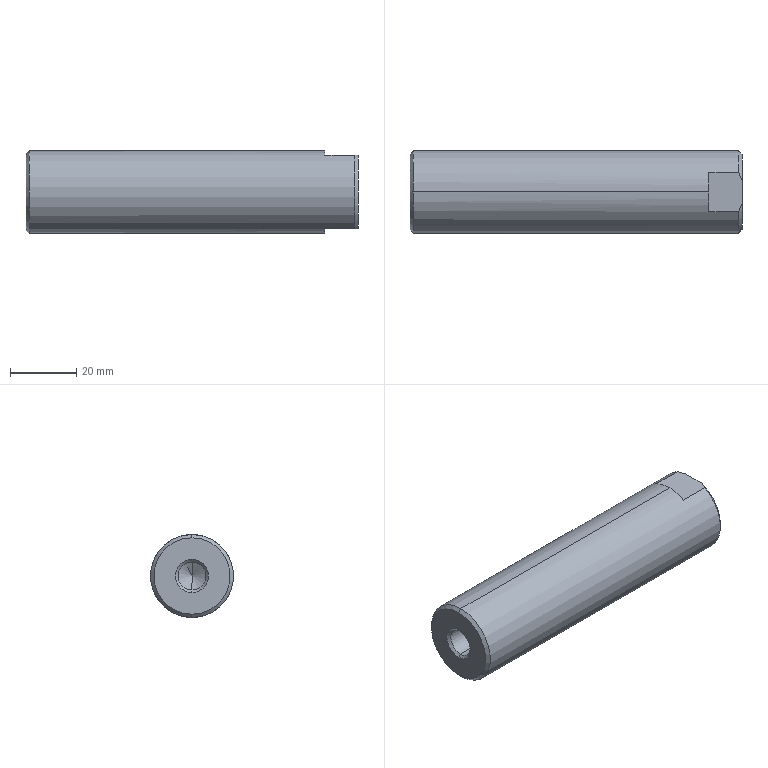Part | STEP file | Part 2 | 1 solid | 18 faces | box 100 x 25 x 25 mm | volume 47263 mm3 | cone 8 | plane 6 | cylinder 4 | commonest cylinder face diameters 8.376 x2 25 x2
STEP:
#1=CARTESIAN_POINT('',(0.,0.,0.));
#2=DIRECTION('',(0.,0.,1.));
#3=DIRECTION('',(1.,0.,0.));
#4=AXIS2_PLACEMENT_3D('',#1,#2,#3);
#5=CARTESIAN_POINT('',(0.812,0.,4.188));
#6=VERTEX_POINT('',#5);
#7=CARTESIAN_POINT('',(0.,0.,5.));
#8=VERTEX_POINT('',#7);
#9=CARTESIAN_POINT('',(0.812,0.,4.188));
#10=DIRECTION('',(-0.7071,0.,0.7071));
#11=VECTOR('',#10,1.);
#12=LINE('',#9,#11);
#13=CARTESIAN_POINT('',(0.812,0.,0.));
#14=DIRECTION('',(-1.,0.,0.));
#15=DIRECTION('',(0.,0.,1.));
#16=AXIS2_PLACEMENT_3D('',#13,#14,#15);
#17=CONICAL_SURFACE('',#16,4.188,0.7854);
#18=CARTESIAN_POINT('',(6.283,0.));
#19=DIRECTION('',(0.,1.));
#20=VECTOR('',#19,1.);
#21=LINE('',#18,#20);
#22=(GEOMETRIC_REPRESENTATION_CONTEXT(2)PARAMETRIC_REPRESENTATION_CONTEXT()REPRESENTATION_CONTEXT('',''));
#23=DEFINITIONAL_REPRESENTATION('',(#21),#22);
#24=PCURVE('',#17,#23);
#25=CARTESIAN_POINT('',(0.812,0.,0.));
#26=DIRECTION('',(-1.,0.,0.));
#27=DIRECTION('',(0.,0.,1.));
#28=AXIS2_PLACEMENT_3D('',#25,#26,#27);
#29=CONICAL_SURFACE('',#28,4.188,0.7854);
#30=CARTESIAN_POINT('',(0.,0.));
#31=DIRECTION('',(0.,1.));
#32=VECTOR('',#31,1.);
#33=LINE('',#30,#32);
#34=(GEOMETRIC_REPRESENTATION_CONTEXT(2)PARAMETRIC_REPRESENTATION_CONTEXT()REPRESENTATION_CONTEXT('',''));
#35=DEFINITIONAL_REPRESENTATION('',(#33),#34);
#36=PCURVE('',#29,#35);
#37=SURFACE_CURVE('',#12,(#24,#36),.PCURVE_S1.);
#38=EDGE_CURVE('',#6,#8,#37,.T.);
#39=ORIENTED_EDGE('',*,*,#38,.T.);
#40=CARTESIAN_POINT('',(0.,0.,-5.));
#41=VERTEX_POINT('',#40);
#42=CARTESIAN_POINT('',(0.,0.,0.));
#43=DIRECTION('',(1.,0.,0.));
#44=DIRECTION('',(0.,0.,1.));
#45=AXIS2_PLACEMENT_3D('',#42,#43,#44);
#46=CIRCLE('',#45,5.);
#47=CARTESIAN_POINT('',(6.283,0.812));
#48=DIRECTION('',(-1.,0.));
#49=VECTOR('',#48,1.);
#50=LINE('',#47,#49);
#51=(GEOMETRIC_REPRESENTATION_CONTEXT(2)PARAMETRIC_REPRESENTATION_CONTEXT()REPRESENTATION_CONTEXT('',''));
#52=DEFINITIONAL_REPRESENTATION('',(#50),#51);
#53=PCURVE('',#17,#52);
#54=CARTESIAN_POINT('',(0.,12.5,0.));
#55=DIRECTION('',(-1.,0.,0.));
#56=DIRECTION('',(0.,0.,1.));
#57=AXIS2_PLACEMENT_3D('',#54,#55,#56);
#58=PLANE('',#57);
#59=CARTESIAN_POINT('',(5.,-12.5));
#60=CARTESIAN_POINT('',(5.,-21.16));
#61=CARTESIAN_POINT('',(-2.5,-16.83));
#62=CARTESIAN_POINT('',(-10.,-12.5));
#63=CARTESIAN_POINT('',(-2.5,-8.17));
#64=CARTESIAN_POINT('',(5.,-3.84));
#65=CARTESIAN_POINT('',(5.,-12.5));
#66=(BOUNDED_CURVE()B_SPLINE_CURVE(2,(#59,#60,#61,#62,#63,#64,#65),.UNSPECIFIED.,.T.,.F.)B_SPLINE_CURVE_WITH_KNOTS((1,2,2,2,2,1),(-2.094,0.,2.094,4.189,6.283,8.378),.UNSPECIFIED.)CURVE()GEOMETRIC_REPRESENTATION_ITEM()RATIONAL_B_SPLINE_CURVE((1.,0.5,1.,0.5,1.,0.5,1.))REPRESENTATION_ITEM(''));
#67=(GEOMETRIC_REPRESENTATION_CONTEXT(2)PARAMETRIC_REPRESENTATION_CONTEXT()REPRESENTATION_CONTEXT('',''));
#68=DEFINITIONAL_REPRESENTATION('',(#66),#67);
#69=PCURVE('',#58,#68);
#70=SURFACE_CURVE('',#46,(#53,#69),.PCURVE_S1.);
#71=EDGE_CURVE('',#8,#41,#70,.T.);
#72=ORIENTED_EDGE('',*,*,#71,.T.);
#73=CARTESIAN_POINT('',(0.812,0.,-4.188));
#74=VERTEX_POINT('',#73);
#75=CARTESIAN_POINT('',(0.812,0.,-4.188));
#76=DIRECTION('',(-0.7071,0.,-0.7071));
#77=VECTOR('',#76,1.);
#78=LINE('',#75,#77);
#79=CARTESIAN_POINT('',(3.142,0.));
#80=DIRECTION('',(0.,1.));
#81=VECTOR('',#80,1.);
#82=LINE('',#79,#81);
#83=(GEOMETRIC_REPRESENTATION_CONTEXT(2)PARAMETRIC_REPRESENTATION_CONTEXT()REPRESENTATION_CONTEXT('',''));
#84=DEFINITIONAL_REPRESENTATION('',(#82),#83);
#85=PCURVE('',#17,#84);
#86=CARTESIAN_POINT('',(3.142,0.));
#87=DIRECTION('',(0.,1.));
#88=VECTOR('',#87,1.);
#89=LINE('',#86,#88);
#90=(GEOMETRIC_REPRESENTATION_CONTEXT(2)PARAMETRIC_REPRESENTATION_CONTEXT()REPRESENTATION_CONTEXT('',''));
#91=DEFINITIONAL_REPRESENTATION('',(#89),#90);
#92=PCURVE('',#29,#91);
#93=SURFACE_CURVE('',#78,(#85,#92),.PCURVE_S1.);
#94=EDGE_CURVE('',#74,#41,#93,.T.);
#95=ORIENTED_EDGE('',*,*,#94,.F.);
#96=CARTESIAN_POINT('',(0.812,0.,0.));
#97=DIRECTION('',(-1.,0.,0.));
#98=DIRECTION('',(0.,0.,1.));
#99=AXIS2_PLACEMENT_3D('',#96,#97,#98);
#100=CIRCLE('',#99,4.188);
#101=CARTESIAN_POINT('',(0.,0.));
#102=DIRECTION('',(1.,0.));
#103=VECTOR('',#102,1.);
#104=LINE('',#101,#103);
#105=(GEOMETRIC_REPRESENTATION_CONTEXT(2)PARAMETRIC_REPRESENTATION_CONTEXT()REPRESENTATION_CONTEXT('',''));
#106=DEFINITIONAL_REPRESENTATION('',(#104),#105);
#107=PCURVE('',#17,#106);
#108=CARTESIAN_POINT('',(0.,0.,0.));
#109=DIRECTION('',(-1.,0.,0.));
#110=DIRECTION('',(0.,0.,1.));
#111=AXIS2_PLACEMENT_3D('',#108,#109,#110);
#112=CYLINDRICAL_SURFACE('',#111,4.188);
#113=CARTESIAN_POINT('',(0.,-0.812));
#114=DIRECTION('',(1.,0.));
#115=VECTOR('',#114,1.);
#116=LINE('',#113,#115);
#117=(GEOMETRIC_REPRESENTATION_CONTEXT(2)PARAMETRIC_REPRESENTATION_CONTEXT()REPRESENTATION_CONTEXT('',''));
#118=DEFINITIONAL_REPRESENTATION('',(#116),#117);
#119=PCURVE('',#112,#118);
#120=SURFACE_CURVE('',#100,(#107,#119),.PCURVE_S1.);
#121=EDGE_CURVE('',#74,#6,#120,.T.);
#122=ORIENTED_EDGE('',*,*,#121,.T.);
#123=EDGE_LOOP('',(#39,#72,#95,#122));
#124=FACE_BOUND('',#123,.F.);
#125=ADVANCED_FACE('',(#124),#17,.F.);
#126=CARTESIAN_POINT('',(0.,0.,11.5));
#127=VERTEX_POINT('',#126);
#128=CARTESIAN_POINT('',(0.,0.,-11.5));
#129=VERTEX_POINT('',#128);
#130=CARTESIAN_POINT('',(0.,0.,0.));
#131=DIRECTION('',(-1.,0.,0.));
#132=DIRECTION('',(0.,0.,1.));
#133=AXIS2_PLACEMENT_3D('',#130,#131,#132);
#134=CIRCLE('',#133,11.5);
#135=CARTESIAN_POINT('',(1.,0.,0.));
#136=DIRECTION('',(1.,0.,0.));
#137=DIRECTION('',(0.,0.,-1.));
#138=AXIS2_PLACEMENT_3D('',#135,#136,#137);
#139=CONICAL_SURFACE('',#138,12.5,0.7854);
#140=CARTESIAN_POINT('',(3.142,-1.));
#141=DIRECTION('',(-1.,0.));
#142=VECTOR('',#141,1.);
#143=LINE('',#140,#142);
#144=(GEOMETRIC_REPRESENTATION_CONTEXT(2)PARAMETRIC_REPRESENTATION_CONTEXT()REPRESENTATION_CONTEXT('',''));
#145=DEFINITIONAL_REPRESENTATION('',(#143),#144);
#146=PCURVE('',#139,#145);
#147=CARTESIAN_POINT('',(0.,-12.5));
#148=DIRECTION('',(1.,0.));
#149=AXIS2_PLACEMENT_2D('',#147,#148);
#150=CIRCLE('',#149,11.5);
#151=(GEOMETRIC_REPRESENTATION_CONTEXT(2)PARAMETRIC_REPRESENTATION_CONTEXT()REPRESENTATION_CONTEXT('',''));
#152=DEFINITIONAL_REPRESENTATION('',(#150),#151);
#153=PCURVE('',#58,#152);
#154=SURFACE_CURVE('',#134,(#146,#153),.PCURVE_S1.);
#155=EDGE_CURVE('',#127,#129,#154,.T.);
#156=ORIENTED_EDGE('',*,*,#155,.F.);
#157=CARTESIAN_POINT('',(1.,0.,12.5));
#158=VERTEX_POINT('',#157);
#159=CARTESIAN_POINT('',(1.,0.,12.5));
#160=DIRECTION('',(0.7071,0.,0.7071));
#161=VECTOR('',#160,1.);
#162=LINE('',#159,#161);
#163=CARTESIAN_POINT('',(3.142,0.));
#164=DIRECTION('',(0.,1.));
#165=VECTOR('',#164,1.);
#166=LINE('',#163,#165);
#167=(GEOMETRIC_REPRESENTATION_CONTEXT(2)PARAMETRIC_REPRESENTATION_CONTEXT()REPRESENTATION_CONTEXT('',''));
#168=DEFINITIONAL_REPRESENTATION('',(#166),#167);
#169=PCURVE('',#139,#168);
#170=CARTESIAN_POINT('',(1.,0.,0.));
#171=DIRECTION('',(1.,0.,0.));
#172=DIRECTION('',(0.,0.,-1.));
#173=AXIS2_PLACEMENT_3D('',#170,#171,#172);
#174=CONICAL_SURFACE('',#173,12.5,0.7854);
#175=CARTESIAN_POINT('',(3.142,0.));
#176=DIRECTION('',(0.,1.));
#177=VECTOR('',#176,1.);
#178=LINE('',#175,#177);
#179=(GEOMETRIC_REPRESENTATION_CONTEXT(2)PARAMETRIC_REPRESENTATION_CONTEXT()REPRESENTATION_CONTEXT('',''));
#180=DEFINITIONAL_REPRESENTATION('',(#178),#179);
#181=PCURVE('',#174,#180);
#182=SURFACE_CURVE('',#162,(#169,#181),.PCURVE_S1.);
#183=EDGE_CURVE('',#127,#158,#182,.T.);
#184=ORIENTED_EDGE('',*,*,#183,.T.);
#185=CARTESIAN_POINT('',(1.,0.,-12.5));
#186=VERTEX_POINT('',#185);
#187=CARTESIAN_POINT('',(1.,0.,0.));
#188=DIRECTION('',(1.,0.,0.));
#189=DIRECTION('',(0.,0.,1.));
#190=AXIS2_PLACEMENT_3D('',#187,#188,#189);
#191=CIRCLE('',#190,12.5);
#192=CARTESIAN_POINT('',(-3.142,0.));
#193=DIRECTION('',(1.,0.));
#194=VECTOR('',#193,1.);
#195=LINE('',#192,#194);
#196=(GEOMETRIC_REPRESENTATION_CONTEXT(2)PARAMETRIC_REPRESENTATION_CONTEXT()REPRESENTATION_CONTEXT('',''));
#197=DEFINITIONAL_REPRESENTATION('',(#195),#196);
#198=PCURVE('',#139,#197);
#199=CARTESIAN_POINT('',(0.,0.,0.));
#200=DIRECTION('',(1.,0.,0.));
#201=DIRECTION('',(0.,0.,-1.));
#202=AXIS2_PLACEMENT_3D('',#199,#200,#201);
#203=CYLINDRICAL_SURFACE('',#202,12.5);
#204=CARTESIAN_POINT('',(-3.142,1.));
#205=DIRECTION('',(1.,0.));
#206=VECTOR('',#205,1.);
#207=LINE('',#204,#206);
#208=(GEOMETRIC_REPRESENTATION_CONTEXT(2)PARAMETRIC_REPRESENTATION_CONTEXT()REPRESENTATION_CONTEXT('',''));
#209=DEFINITIONAL_REPRESENTATION('',(#207),#208);
#210=PCURVE('',#203,#209);
#211=SURFACE_CURVE('',#191,(#198,#210),.PCURVE_S1.);
#212=EDGE_CURVE('',#186,#158,#211,.T.);
#213=ORIENTED_EDGE('',*,*,#212,.F.);
#214=CARTESIAN_POINT('',(1.,0.,-12.5));
#215=DIRECTION('',(0.7071,0.,-0.7071));
#216=VECTOR('',#215,1.);
#217=LINE('',#214,#216);
#218=CARTESIAN_POINT('',(0.,0.));
#219=DIRECTION('',(0.,1.));
#220=VECTOR('',#219,1.);
#221=LINE('',#218,#220);
#222=(GEOMETRIC_REPRESENTATION_CONTEXT(2)PARAMETRIC_REPRESENTATION_CONTEXT()REPRESENTATION_CONTEXT('',''));
#223=DEFINITIONAL_REPRESENTATION('',(#221),#222);
#224=PCURVE('',#139,#223);
#225=CARTESIAN_POINT('',(6.283,0.));
#226=DIRECTION('',(0.,1.));
#227=VECTOR('',#226,1.);
#228=LINE('',#225,#227);
#229=(GEOMETRIC_REPRESENTATION_CONTEXT(2)PARAMETRIC_REPRESENTATION_CONTEXT()REPRESENTATION_CONTEXT('',''));
#230=DEFINITIONAL_REPRESENTATION('',(#228),#229);
#231=PCURVE('',#174,#230);
#232=SURFACE_CURVE('',#217,(#224,#231),.PCURVE_S1.);
#233=EDGE_CURVE('',#129,#186,#232,.T.);
#234=ORIENTED_EDGE('',*,*,#233,.F.);
#235=EDGE_LOOP('',(#156,#184,#213,#234));
#236=FACE_BOUND('',#235,.T.);
#237=ADVANCED_FACE('',(#236),#139,.T.);
#238=CARTESIAN_POINT('',(26.582,0.,4.188));
#239=VERTEX_POINT('',#238);
#240=CARTESIAN_POINT('',(0.,0.,4.188));
#241=DIRECTION('',(-1.,0.,0.));
#242=VECTOR('',#241,1.);
#243=LINE('',#240,#242);
#244=CARTESIAN_POINT('',(6.283,0.));
#245=DIRECTION('',(0.,1.));
#246=VECTOR('',#245,1.);
#247=LINE('',#244,#246);
#248=(GEOMETRIC_REPRESENTATION_CONTEXT(2)PARAMETRIC_REPRESENTATION_CONTEXT()REPRESENTATION_CONTEXT('',''));
#249=DEFINITIONAL_REPRESENTATION('',(#247),#248);
#250=PCURVE('',#112,#249);
#251=CARTESIAN_POINT('',(0.,0.,0.));
#252=DIRECTION('',(-1.,0.,0.));
#253=DIRECTION('',(0.,0.,1.));
#254=AXIS2_PLACEMENT_3D('',#251,#252,#253);
#255=CYLINDRICAL_SURFACE('',#254,4.188);
#256=CARTESIAN_POINT('',(0.,0.));
#257=DIRECTION('',(0.,1.));
#258=VECTOR('',#257,1.);
#259=LINE('',#256,#258);
#260=(GEOMETRIC_REPRESENTATION_CONTEXT(2)PARAMETRIC_REPRESENTATION_CONTEXT()REPRESENTATION_CONTEXT('',''));
#261=DEFINITIONAL_REPRESENTATION('',(#259),#260);
#262=PCURVE('',#255,#261);
#263=SURFACE_CURVE('',#243,(#250,#262),.PCURVE_S1.);
#264=EDGE_CURVE('',#239,#6,#263,.T.);
#265=ORIENTED_EDGE('',*,*,#264,.T.);
#266=ORIENTED_EDGE('',*,*,#121,.F.);
#267=CARTESIAN_POINT('',(26.582,0.,-4.188));
#268=VERTEX_POINT('',#267);
#269=CARTESIAN_POINT('',(0.,0.,-4.188));
#270=DIRECTION('',(-1.,0.,0.));
#271=VECTOR('',#270,1.);
#272=LINE('',#269,#271);
#273=CARTESIAN_POINT('',(3.142,0.));
#274=DIRECTION('',(0.,1.));
#275=VECTOR('',#274,1.);
#276=LINE('',#273,#275);
#277=(GEOMETRIC_REPRESENTATION_CONTEXT(2)PARAMETRIC_REPRESENTATION_CONTEXT()REPRESENTATION_CONTEXT('',''));
#278=DEFINITIONAL_REPRESENTATION('',(#276),#277);
#279=PCURVE('',#112,#278);
#280=CARTESIAN_POINT('',(3.142,0.));
#281=DIRECTION('',(0.,1.));
#282=VECTOR('',#281,1.);
#283=LINE('',#280,#282);
#284=(GEOMETRIC_REPRESENTATION_CONTEXT(2)PARAMETRIC_REPRESENTATION_CONTEXT()REPRESENTATION_CONTEXT('',''));
#285=DEFINITIONAL_REPRESENTATION('',(#283),#284);
#286=PCURVE('',#255,#285);
#287=SURFACE_CURVE('',#272,(#279,#286),.PCURVE_S1.);
#288=EDGE_CURVE('',#268,#74,#287,.T.);
#289=ORIENTED_EDGE('',*,*,#288,.F.);
#290=CARTESIAN_POINT('',(26.582,0.,0.));
#291=DIRECTION('',(-1.,0.,0.));
#292=DIRECTION('',(0.,0.,1.));
#293=AXIS2_PLACEMENT_3D('',#290,#291,#292);
#294=CIRCLE('',#293,4.188);
#295=CARTESIAN_POINT('',(0.,-26.582));
#296=DIRECTION('',(1.,0.));
#297=VECTOR('',#296,1.);
#298=LINE('',#295,#297);
#299=(GEOMETRIC_REPRESENTATION_CONTEXT(2)PARAMETRIC_REPRESENTATION_CONTEXT()REPRESENTATION_CONTEXT('',''));
#300=DEFINITIONAL_REPRESENTATION('',(#298),#299);
#301=PCURVE('',#112,#300);
#302=CARTESIAN_POINT('',(26.582,0.,0.));
#303=DIRECTION('',(-1.,0.,0.));
#304=DIRECTION('',(0.,0.,1.));
#305=AXIS2_PLACEMENT_3D('',#302,#303,#304);
#306=CONICAL_SURFACE('',#305,4.188,1.047);
#307=CARTESIAN_POINT('',(0.,0.));
#308=DIRECTION('',(1.,0.));
#309=VECTOR('',#308,1.);
#310=LINE('',#307,#309);
#311=(GEOMETRIC_REPRESENTATION_CONTEXT(2)PARAMETRIC_REPRESENTATION_CONTEXT()REPRESENTATION_CONTEXT('',''));
#312=DEFINITIONAL_REPRESENTATION('',(#310),#311);
#313=PCURVE('',#306,#312);
#314=SURFACE_CURVE('',#294,(#301,#313),.PCURVE_S1.);
#315=EDGE_CURVE('',#268,#239,#314,.T.);
#316=ORIENTED_EDGE('',*,*,#315,.T.);
#317=EDGE_LOOP('',(#265,#266,#289,#316));
#318=FACE_BOUND('',#317,.F.);
#319=ADVANCED_FACE('',(#318),#112,.F.);
#320=ORIENTED_EDGE('',*,*,#315,.F.);
#321=CARTESIAN_POINT('',(29.,0.,0.));
#322=VERTEX_POINT('',#321);
#323=CARTESIAN_POINT('',(26.582,0.,-4.188));
#324=DIRECTION('',(-0.5,0.,-0.866));
#325=VECTOR('',#324,1.);
#326=LINE('',#323,#325);
#327=CARTESIAN_POINT('',(3.142,-2.418));
#328=CARTESIAN_POINT('',(3.142,-2.381));
#329=CARTESIAN_POINT('',(3.142,-2.308));
#330=CARTESIAN_POINT('',(3.142,-2.198));
#331=CARTESIAN_POINT('',(3.142,-2.088));
#332=CARTESIAN_POINT('',(3.142,-1.978));
#333=CARTESIAN_POINT('',(3.142,-1.868));
#334=CARTESIAN_POINT('',(3.142,-1.759));
#335=CARTESIAN_POINT('',(3.142,-1.649));
#336=CARTESIAN_POINT('',(3.142,-1.539));
#337=CARTESIAN_POINT('',(3.142,-1.429));
#338=CARTESIAN_POINT('',(3.142,-1.319));
#339=CARTESIAN_POINT('',(3.142,-1.209));
#340=CARTESIAN_POINT('',(3.142,-1.099));
#341=CARTESIAN_POINT('',(3.142,-0.9892));
#342=CARTESIAN_POINT('',(3.142,-0.8793));
#343=CARTESIAN_POINT('',(3.142,-0.7693));
#344=CARTESIAN_POINT('',(3.142,-0.6594));
#345=CARTESIAN_POINT('',(3.142,-0.5495));
#346=CARTESIAN_POINT('',(3.142,-0.4396));
#347=CARTESIAN_POINT('',(3.142,-0.3297));
#348=CARTESIAN_POINT('',(3.142,-0.2198));
#349=CARTESIAN_POINT('',(3.142,-0.1099));
#350=CARTESIAN_POINT('',(3.142,-0.03664));
#351=CARTESIAN_POINT('',(3.142,0.));
#352=B_SPLINE_CURVE_WITH_KNOTS('',3,(#327,#328,#329,#330,#331,#332,#333,#334,#335,#336,#337,#338,#339,#340,#341,#342,#343,#344,#345,#346,#347,#348,#349,#350,#351),.UNSPECIFIED.,.F.,.F.,(4,1,1,1,1,1,1,1,1,1,1,1,1,1,1,1,1,1,1,1,1,1,4),(-4.836,-4.616,-4.396,-4.176,-3.957,-3.737,-3.517,-3.297,-3.077,-2.858,-2.638,-2.418,-2.198,-1.978,-1.759,-1.539,-1.319,-1.099,-0.8793,-0.6594,-0.4396,-0.2198,0.),.QUASI_UNIFORM_KNOTS.);
#353=(GEOMETRIC_REPRESENTATION_CONTEXT(2)PARAMETRIC_REPRESENTATION_CONTEXT()REPRESENTATION_CONTEXT('',''));
#354=DEFINITIONAL_REPRESENTATION('',(#352),#353);
#355=PCURVE('',#306,#354);
#356=CARTESIAN_POINT('',(26.582,0.,0.));
#357=DIRECTION('',(-1.,0.,0.));
#358=DIRECTION('',(0.,0.,1.));
#359=AXIS2_PLACEMENT_3D('',#356,#357,#358);
#360=CONICAL_SURFACE('',#359,4.188,1.047);
#361=CARTESIAN_POINT('',(3.142,-2.418));
#362=CARTESIAN_POINT('',(3.142,-2.381));
#363=CARTESIAN_POINT('',(3.142,-2.308));
#364=CARTESIAN_POINT('',(3.142,-2.198));
#365=CARTESIAN_POINT('',(3.142,-2.088));
#366=CARTESIAN_POINT('',(3.142,-1.978));
#367=CARTESIAN_POINT('',(3.142,-1.868));
#368=CARTESIAN_POINT('',(3.142,-1.759));
#369=CARTESIAN_POINT('',(3.142,-1.649));
#370=CARTESIAN_POINT('',(3.142,-1.539));
#371=CARTESIAN_POINT('',(3.142,-1.429));
#372=CARTESIAN_POINT('',(3.142,-1.319));
#373=CARTESIAN_POINT('',(3.142,-1.209));
#374=CARTESIAN_POINT('',(3.142,-1.099));
#375=CARTESIAN_POINT('',(3.142,-0.9892));
#376=CARTESIAN_POINT('',(3.142,-0.8793));
#377=CARTESIAN_POINT('',(3.142,-0.7693));
#378=CARTESIAN_POINT('',(3.142,-0.6594));
#379=CARTESIAN_POINT('',(3.142,-0.5495));
#380=CARTESIAN_POINT('',(3.142,-0.4396));
#381=CARTESIAN_POINT('',(3.142,-0.3297));
#382=CARTESIAN_POINT('',(3.142,-0.2198));
#383=CARTESIAN_POINT('',(3.142,-0.1099));
#384=CARTESIAN_POINT('',(3.142,-0.03664));
#385=CARTESIAN_POINT('',(3.142,0.));
#386=B_SPLINE_CURVE_WITH_KNOTS('',3,(#361,#362,#363,#364,#365,#366,#367,#368,#369,#370,#371,#372,#373,#374,#375,#376,#377,#378,#379,#380,#381,#382,#383,#384,#385),.UNSPECIFIED.,.F.,.F.,(4,1,1,1,1,1,1,1,1,1,1,1,1,1,1,1,1,1,1,1,1,1,4),(-4.836,-4.616,-4.396,-4.176,-3.957,-3.737,-3.517,-3.297,-3.077,-2.858,-2.638,-2.418,-2.198,-1.978,-1.759,-1.539,-1.319,-1.099,-0.8793,-0.6594,-0.4396,-0.2198,0.),.QUASI_UNIFORM_KNOTS.);
#387=(GEOMETRIC_REPRESENTATION_CONTEXT(2)PARAMETRIC_REPRESENTATION_CONTEXT()REPRESENTATION_CONTEXT('',''));
#388=DEFINITIONAL_REPRESENTATION('',(#386),#387);
#389=PCURVE('',#360,#388);
#390=SURFACE_CURVE('',#326,(#355,#389),.PCURVE_S1.);
#391=EDGE_CURVE('',#322,#268,#390,.T.);
#392=ORIENTED_EDGE('',*,*,#391,.F.);
#393=CARTESIAN_POINT('',(26.582,0.,4.188));
#394=DIRECTION('',(-0.5,0.,0.866));
#395=VECTOR('',#394,1.);
#396=LINE('',#393,#395);
#397=CARTESIAN_POINT('',(6.283,-2.418));
#398=CARTESIAN_POINT('',(6.283,-2.381));
#399=CARTESIAN_POINT('',(6.283,-2.308));
#400=CARTESIAN_POINT('',(6.283,-2.198));
#401=CARTESIAN_POINT('',(6.283,-2.088));
#402=CARTESIAN_POINT('',(6.283,-1.978));
#403=CARTESIAN_POINT('',(6.283,-1.868));
#404=CARTESIAN_POINT('',(6.283,-1.759));
#405=CARTESIAN_POINT('',(6.283,-1.649));
#406=CARTESIAN_POINT('',(6.283,-1.539));
#407=CARTESIAN_POINT('',(6.283,-1.429));
#408=CARTESIAN_POINT('',(6.283,-1.319));
#409=CARTESIAN_POINT('',(6.283,-1.209));
#410=CARTESIAN_POINT('',(6.283,-1.099));
#411=CARTESIAN_POINT('',(6.283,-0.9892));
#412=CARTESIAN_POINT('',(6.283,-0.8793));
#413=CARTESIAN_POINT('',(6.283,-0.7693));
#414=CARTESIAN_POINT('',(6.283,-0.6594));
#415=CARTESIAN_POINT('',(6.283,-0.5495));
#416=CARTESIAN_POINT('',(6.283,-0.4396));
#417=CARTESIAN_POINT('',(6.283,-0.3297));
#418=CARTESIAN_POINT('',(6.283,-0.2198));
#419=CARTESIAN_POINT('',(6.283,-0.1099));
#420=CARTESIAN_POINT('',(6.283,-0.03664));
#421=CARTESIAN_POINT('',(6.283,0.));
#422=B_SPLINE_CURVE_WITH_KNOTS('',3,(#397,#398,#399,#400,#401,#402,#403,#404,#405,#406,#407,#408,#409,#410,#411,#412,#413,#414,#415,#416,#417,#418,#419,#420,#421),.UNSPECIFIED.,.F.,.F.,(4,1,1,1,1,1,1,1,1,1,1,1,1,1,1,1,1,1,1,1,1,1,4),(-4.836,-4.616,-4.396,-4.176,-3.957,-3.737,-3.517,-3.297,-3.077,-2.858,-2.638,-2.418,-2.198,-1.978,-1.759,-1.539,-1.319,-1.099,-0.8793,-0.6594,-0.4396,-0.2198,0.),.QUASI_UNIFORM_KNOTS.);
#423=(GEOMETRIC_REPRESENTATION_CONTEXT(2)PARAMETRIC_REPRESENTATION_CONTEXT()REPRESENTATION_CONTEXT('',''));
#424=DEFINITIONAL_REPRESENTATION('',(#422),#423);
#425=PCURVE('',#306,#424);
#426=CARTESIAN_POINT('',(0.,-2.418));
#427=CARTESIAN_POINT('',(0.,-2.381));
#428=CARTESIAN_POINT('',(0.,-2.308));
#429=CARTESIAN_POINT('',(0.,-2.198));
#430=CARTESIAN_POINT('',(0.,-2.088));
#431=CARTESIAN_POINT('',(0.,-1.978));
#432=CARTESIAN_POINT('',(0.,-1.868));
#433=CARTESIAN_POINT('',(0.,-1.759));
#434=CARTESIAN_POINT('',(0.,-1.649));
#435=CARTESIAN_POINT('',(0.,-1.539));
#436=CARTESIAN_POINT('',(0.,-1.429));
#437=CARTESIAN_POINT('',(0.,-1.319));
#438=CARTESIAN_POINT('',(0.,-1.209));
#439=CARTESIAN_POINT('',(0.,-1.099));
#440=CARTESIAN_POINT('',(0.,-0.9892));
#441=CARTESIAN_POINT('',(0.,-0.8793));
#442=CARTESIAN_POINT('',(0.,-0.7693));
#443=CARTESIAN_POINT('',(0.,-0.6594));
#444=CARTESIAN_POINT('',(0.,-0.5495));
#445=CARTESIAN_POINT('',(0.,-0.4396));
#446=CARTESIAN_POINT('',(0.,-0.3297));
#447=CARTESIAN_POINT('',(0.,-0.2198));
#448=CARTESIAN_POINT('',(0.,-0.1099));
#449=CARTESIAN_POINT('',(0.,-0.03664));
#450=CARTESIAN_POINT('',(0.,0.));
#451=B_SPLINE_CURVE_WITH_KNOTS('',3,(#426,#427,#428,#429,#430,#431,#432,#433,#434,#435,#436,#437,#438,#439,#440,#441,#442,#443,#444,#445,#446,#447,#448,#449,#450),.UNSPECIFIED.,.F.,.F.,(4,1,1,1,1,1,1,1,1,1,1,1,1,1,1,1,1,1,1,1,1,1,4),(-4.836,-4.616,-4.396,-4.176,-3.957,-3.737,-3.517,-3.297,-3.077,-2.858,-2.638,-2.418,-2.198,-1.978,-1.759,-1.539,-1.319,-1.099,-0.8793,-0.6594,-0.4396,-0.2198,0.),.QUASI_UNIFORM_KNOTS.);
#452=(GEOMETRIC_REPRESENTATION_CONTEXT(2)PARAMETRIC_REPRESENTATION_CONTEXT()REPRESENTATION_CONTEXT('',''));
#453=DEFINITIONAL_REPRESENTATION('',(#451),#452);
#454=PCURVE('',#360,#453);
#455=SURFACE_CURVE('',#396,(#425,#454),.PCURVE_S1.);
#456=EDGE_CURVE('',#322,#239,#455,.T.);
#457=ORIENTED_EDGE('',*,*,#456,.T.);
#458=EDGE_LOOP('',(#320,#392,#457));
#459=FACE_BOUND('',#458,.F.);
#460=ADVANCED_FACE('',(#459),#306,.F.);
#461=ORIENTED_EDGE('',*,*,#212,.T.);
#462=CARTESIAN_POINT('',(90.,0.,12.5));
#463=VERTEX_POINT('',#462);
#464=CARTESIAN_POINT('',(0.,0.,12.5));
#465=DIRECTION('',(1.,0.,0.));
#466=VECTOR('',#465,1.);
#467=LINE('',#464,#466);
#468=CARTESIAN_POINT('',(3.142,0.));
#469=DIRECTION('',(0.,1.));
#470=VECTOR('',#469,1.);
#471=LINE('',#468,#470);
#472=(GEOMETRIC_REPRESENTATION_CONTEXT(2)PARAMETRIC_REPRESENTATION_CONTEXT()REPRESENTATION_CONTEXT('',''));
#473=DEFINITIONAL_REPRESENTATION('',(#471),#472);
#474=PCURVE('',#203,#473);
#475=CARTESIAN_POINT('',(0.,0.,0.));
#476=DIRECTION('',(1.,0.,0.));
#477=DIRECTION('',(0.,0.,-1.));
#478=AXIS2_PLACEMENT_3D('',#475,#476,#477);
#479=CYLINDRICAL_SURFACE('',#478,12.5);
#480=CARTESIAN_POINT('',(3.142,0.));
#481=DIRECTION('',(0.,1.));
#482=VECTOR('',#481,1.);
#483=LINE('',#480,#482);
#484=(GEOMETRIC_REPRESENTATION_CONTEXT(2)PARAMETRIC_REPRESENTATION_CONTEXT()REPRESENTATION_CONTEXT('',''));
#485=DEFINITIONAL_REPRESENTATION('',(#483),#484);
#486=PCURVE('',#479,#485);
#487=SURFACE_CURVE('',#467,(#474,#486),.PCURVE_S1.);
#488=EDGE_CURVE('',#158,#463,#487,.T.);
#489=ORIENTED_EDGE('',*,*,#488,.T.);
#490=CARTESIAN_POINT('',(90.,5.937,11.));
#491=VERTEX_POINT('',#490);
#492=CARTESIAN_POINT('',(90.,0.,0.));
#493=DIRECTION('',(1.,0.,0.));
#494=DIRECTION('',(0.,0.,-1.));
#495=AXIS2_PLACEMENT_3D('',#492,#493,#494);
#496=CIRCLE('',#495,12.5);
#497=CARTESIAN_POINT('',(0.,90.));
#498=DIRECTION('',(1.,0.));
#499=VECTOR('',#498,1.);
#500=LINE('',#497,#499);
#501=(GEOMETRIC_REPRESENTATION_CONTEXT(2)PARAMETRIC_REPRESENTATION_CONTEXT()REPRESENTATION_CONTEXT('',''));
#502=DEFINITIONAL_REPRESENTATION('',(#500),#501);
#503=PCURVE('',#203,#502);
#504=CARTESIAN_POINT('',(90.,0.,0.));
#505=DIRECTION('',(1.,0.,0.));
#506=DIRECTION('',(0.,0.,-1.));
#507=AXIS2_PLACEMENT_3D('',#504,#505,#506);
#508=PLANE('',#507);
#509=CARTESIAN_POINT('',(0.,0.));
#510=DIRECTION('',(1.,0.));
#511=AXIS2_PLACEMENT_2D('',#509,#510);
#512=CIRCLE('',#511,12.5);
#513=(GEOMETRIC_REPRESENTATION_CONTEXT(2)PARAMETRIC_REPRESENTATION_CONTEXT()REPRESENTATION_CONTEXT('',''));
#514=DEFINITIONAL_REPRESENTATION('',(#512),#513);
#515=PCURVE('',#508,#514);
#516=SURFACE_CURVE('',#496,(#503,#515),.PCURVE_S1.);
#517=EDGE_CURVE('',#491,#463,#516,.T.);
#518=ORIENTED_EDGE('',*,*,#517,.F.);
#519=CARTESIAN_POINT('',(99.,5.937,11.));
#520=VERTEX_POINT('',#519);
#521=CARTESIAN_POINT('',(90.,5.937,11.));
#522=DIRECTION('',(1.,0.,0.));
#523=VECTOR('',#522,1.);
#524=LINE('',#521,#523);
#525=CARTESIAN_POINT('',(2.647,90.));
#526=DIRECTION('',(0.,1.));
#527=VECTOR('',#526,1.);
#528=LINE('',#525,#527);
#529=(GEOMETRIC_REPRESENTATION_CONTEXT(2)PARAMETRIC_REPRESENTATION_CONTEXT()REPRESENTATION_CONTEXT('',''));
#530=DEFINITIONAL_REPRESENTATION('',(#528),#529);
#531=PCURVE('',#203,#530);
#532=CARTESIAN_POINT('',(90.,-5.937,11.));
#533=DIRECTION('',(0.,0.,-1.));
#534=DIRECTION('',(-1.,0.,0.));
#535=AXIS2_PLACEMENT_3D('',#532,#533,#534);
#536=PLANE('',#535);
#537=CARTESIAN_POINT('',(0.,11.874));
#538=DIRECTION('',(-1.,0.));
#539=VECTOR('',#538,1.);
#540=LINE('',#537,#539);
#541=(GEOMETRIC_REPRESENTATION_CONTEXT(2)PARAMETRIC_REPRESENTATION_CONTEXT()REPRESENTATION_CONTEXT('',''));
#542=DEFINITIONAL_REPRESENTATION('',(#540),#541);
#543=PCURVE('',#536,#542);
#544=SURFACE_CURVE('',#524,(#531,#543),.PCURVE_S1.);
#545=EDGE_CURVE('',#491,#520,#544,.T.);
#546=ORIENTED_EDGE('',*,*,#545,.T.);
#547=CARTESIAN_POINT('',(99.,5.937,-11.));
#548=VERTEX_POINT('',#547);
#549=CARTESIAN_POINT('',(99.,0.,0.));
#550=DIRECTION('',(-1.,0.,0.));
#551=DIRECTION('',(0.,0.,-1.));
#552=AXIS2_PLACEMENT_3D('',#549,#550,#551);
#553=CIRCLE('',#552,12.5);
#554=CARTESIAN_POINT('',(6.283,99.));
#555=DIRECTION('',(-1.,0.));
#556=VECTOR('',#555,1.);
#557=LINE('',#554,#556);
#558=(GEOMETRIC_REPRESENTATION_CONTEXT(2)PARAMETRIC_REPRESENTATION_CONTEXT()REPRESENTATION_CONTEXT('',''));
#559=DEFINITIONAL_REPRESENTATION('',(#557),#558);
#560=PCURVE('',#203,#559);
#561=CARTESIAN_POINT('',(100.,0.,0.));
#562=DIRECTION('',(-1.,0.,0.));
#563=DIRECTION('',(0.,0.,1.));
#564=AXIS2_PLACEMENT_3D('',#561,#562,#563);
#565=CONICAL_SURFACE('',#564,11.5,0.7854);
#566=CARTESIAN_POINT('',(-3.142,1.));
#567=DIRECTION('',(1.,0.));
#568=VECTOR('',#567,1.);
#569=LINE('',#566,#568);
#570=(GEOMETRIC_REPRESENTATION_CONTEXT(2)PARAMETRIC_REPRESENTATION_CONTEXT()REPRESENTATION_CONTEXT('',''));
#571=DEFINITIONAL_REPRESENTATION('',(#569),#570);
#572=PCURVE('',#565,#571);
#573=SURFACE_CURVE('',#553,(#560,#572),.PCURVE_S1.);
#574=EDGE_CURVE('',#520,#548,#573,.T.);
#575=ORIENTED_EDGE('',*,*,#574,.T.);
#576=CARTESIAN_POINT('',(90.,5.937,-11.));
#577=VERTEX_POINT('',#576);
#578=CARTESIAN_POINT('',(90.,5.937,-11.));
#579=DIRECTION('',(1.,0.,0.));
#580=VECTOR('',#579,1.);
#581=LINE('',#578,#580);
#582=CARTESIAN_POINT('',(0.4949,90.));
#583=DIRECTION('',(0.,1.));
#584=VECTOR('',#583,1.);
#585=LINE('',#582,#584);
#586=(GEOMETRIC_REPRESENTATION_CONTEXT(2)PARAMETRIC_REPRESENTATION_CONTEXT()REPRESENTATION_CONTEXT('',''));
#587=DEFINITIONAL_REPRESENTATION('',(#585),#586);
#588=PCURVE('',#203,#587);
#589=CARTESIAN_POINT('',(90.,5.937,-11.));
#590=DIRECTION('',(0.,0.,1.));
#591=DIRECTION('',(1.,0.,0.));
#592=AXIS2_PLACEMENT_3D('',#589,#590,#591);
#593=PLANE('',#592);
#594=CARTESIAN_POINT('',(0.,0.));
#595=DIRECTION('',(1.,0.));
#596=VECTOR('',#595,1.);
#597=LINE('',#594,#596);
#598=(GEOMETRIC_REPRESENTATION_CONTEXT(2)PARAMETRIC_REPRESENTATION_CONTEXT()REPRESENTATION_CONTEXT('',''));
#599=DEFINITIONAL_REPRESENTATION('',(#597),#598);
#600=PCURVE('',#593,#599);
#601=SURFACE_CURVE('',#581,(#588,#600),.PCURVE_S1.);
#602=EDGE_CURVE('',#577,#548,#601,.T.);
#603=ORIENTED_EDGE('',*,*,#602,.F.);
#604=CARTESIAN_POINT('',(90.,0.,-12.5));
#605=VERTEX_POINT('',#604);
#606=CARTESIAN_POINT('',(90.,0.,0.));
#607=DIRECTION('',(1.,0.,0.));
#608=DIRECTION('',(0.,0.,-1.));
#609=AXIS2_PLACEMENT_3D('',#606,#607,#608);
#610=CIRCLE('',#609,12.5);
#611=CARTESIAN_POINT('',(0.,90.));
#612=DIRECTION('',(1.,0.));
#613=VECTOR('',#612,1.);
#614=LINE('',#611,#613);
#615=(GEOMETRIC_REPRESENTATION_CONTEXT(2)PARAMETRIC_REPRESENTATION_CONTEXT()REPRESENTATION_CONTEXT('',''));
#616=DEFINITIONAL_REPRESENTATION('',(#614),#615);
#617=PCURVE('',#203,#616);
#618=CARTESIAN_POINT('',(90.,0.,0.));
#619=DIRECTION('',(1.,0.,0.));
#620=DIRECTION('',(0.,0.,-1.));
#621=AXIS2_PLACEMENT_3D('',#618,#619,#620);
#622=PLANE('',#621);
#623=CARTESIAN_POINT('',(0.,0.));
#624=DIRECTION('',(1.,0.));
#625=AXIS2_PLACEMENT_2D('',#623,#624);
#626=CIRCLE('',#625,12.5);
#627=(GEOMETRIC_REPRESENTATION_CONTEXT(2)PARAMETRIC_REPRESENTATION_CONTEXT()REPRESENTATION_CONTEXT('',''));
#628=DEFINITIONAL_REPRESENTATION('',(#626),#627);
#629=PCURVE('',#622,#628);
#630=SURFACE_CURVE('',#610,(#617,#629),.PCURVE_S1.);
#631=EDGE_CURVE('',#605,#577,#630,.T.);
#632=ORIENTED_EDGE('',*,*,#631,.F.);
#633=CARTESIAN_POINT('',(0.,0.,-12.5));
#634=DIRECTION('',(1.,0.,0.));
#635=VECTOR('',#634,1.);
#636=LINE('',#633,#635);
#637=CARTESIAN_POINT('',(0.,0.));
#638=DIRECTION('',(0.,1.));
#639=VECTOR('',#638,1.);
#640=LINE('',#637,#639);
#641=(GEOMETRIC_REPRESENTATION_CONTEXT(2)PARAMETRIC_REPRESENTATION_CONTEXT()REPRESENTATION_CONTEXT('',''));
#642=DEFINITIONAL_REPRESENTATION('',(#640),#641);
#643=PCURVE('',#203,#642);
#644=CARTESIAN_POINT('',(6.283,0.));
#645=DIRECTION('',(0.,1.));
#646=VECTOR('',#645,1.);
#647=LINE('',#644,#646);
#648=(GEOMETRIC_REPRESENTATION_CONTEXT(2)PARAMETRIC_REPRESENTATION_CONTEXT()REPRESENTATION_CONTEXT('',''));
#649=DEFINITIONAL_REPRESENTATION('',(#647),#648);
#650=PCURVE('',#479,#649);
#651=SURFACE_CURVE('',#636,(#643,#650),.PCURVE_S1.);
#652=EDGE_CURVE('',#186,#605,#651,.T.);
#653=ORIENTED_EDGE('',*,*,#652,.F.);
#654=EDGE_LOOP('',(#461,#489,#518,#546,#575,#603,#632,#653));
#655=FACE_BOUND('',#654,.T.);
#656=ADVANCED_FACE('',(#655),#203,.T.);
#657=ORIENTED_EDGE('',*,*,#488,.F.);
#658=CARTESIAN_POINT('',(1.,0.,0.));
#659=DIRECTION('',(1.,0.,0.));
#660=DIRECTION('',(0.,0.,1.));
#661=AXIS2_PLACEMENT_3D('',#658,#659,#660);
#662=CIRCLE('',#661,12.5);
#663=CARTESIAN_POINT('',(3.142,1.));
#664=DIRECTION('',(1.,0.));
#665=VECTOR('',#664,1.);
#666=LINE('',#663,#665);
#667=(GEOMETRIC_REPRESENTATION_CONTEXT(2)PARAMETRIC_REPRESENTATION_CONTEXT()REPRESENTATION_CONTEXT('',''));
#668=DEFINITIONAL_REPRESENTATION('',(#666),#667);
#669=PCURVE('',#479,#668);
#670=CARTESIAN_POINT('',(3.142,0.));
#671=DIRECTION('',(1.,0.));
#672=VECTOR('',#671,1.);
#673=LINE('',#670,#672);
#674=(GEOMETRIC_REPRESENTATION_CONTEXT(2)PARAMETRIC_REPRESENTATION_CONTEXT()REPRESENTATION_CONTEXT('',''));
#675=DEFINITIONAL_REPRESENTATION('',(#673),#674);
#676=PCURVE('',#174,#675);
#677=SURFACE_CURVE('',#662,(#669,#676),.PCURVE_S1.);
#678=EDGE_CURVE('',#158,#186,#677,.T.);
#679=ORIENTED_EDGE('',*,*,#678,.T.);
#680=ORIENTED_EDGE('',*,*,#652,.T.);
#681=CARTESIAN_POINT('',(90.,-5.937,-11.));
#682=VERTEX_POINT('',#681);
#683=CARTESIAN_POINT('',(90.,0.,0.));
#684=DIRECTION('',(1.,0.,0.));
#685=DIRECTION('',(0.,0.,-1.));
#686=AXIS2_PLACEMENT_3D('',#683,#684,#685);
#687=CIRCLE('',#686,12.5);
#688=CARTESIAN_POINT('',(0.,90.));
#689=DIRECTION('',(1.,0.));
#690=VECTOR('',#689,1.);
#691=LINE('',#688,#690);
#692=(GEOMETRIC_REPRESENTATION_CONTEXT(2)PARAMETRIC_REPRESENTATION_CONTEXT()REPRESENTATION_CONTEXT('',''));
#693=DEFINITIONAL_REPRESENTATION('',(#691),#692);
#694=PCURVE('',#479,#693);
#695=CARTESIAN_POINT('',(0.,0.));
#696=DIRECTION('',(1.,0.));
#697=AXIS2_PLACEMENT_2D('',#695,#696);
#698=CIRCLE('',#697,12.5);
#699=(GEOMETRIC_REPRESENTATION_CONTEXT(2)PARAMETRIC_REPRESENTATION_CONTEXT()REPRESENTATION_CONTEXT('',''));
#700=DEFINITIONAL_REPRESENTATION('',(#698),#699);
#701=PCURVE('',#622,#700);
#702=SURFACE_CURVE('',#687,(#694,#701),.PCURVE_S1.);
#703=EDGE_CURVE('',#682,#605,#702,.T.);
#704=ORIENTED_EDGE('',*,*,#703,.F.);
#705=CARTESIAN_POINT('',(99.,-5.937,-11.));
#706=VERTEX_POINT('',#705);
#707=CARTESIAN_POINT('',(90.,-5.937,-11.));
#708=DIRECTION('',(1.,0.,0.));
#709=VECTOR('',#708,1.);
#710=LINE('',#707,#709);
#711=CARTESIAN_POINT('',(5.788,90.));
#712=DIRECTION('',(0.,1.));
#713=VECTOR('',#712,1.);
#714=LINE('',#711,#713);
#715=(GEOMETRIC_REPRESENTATION_CONTEXT(2)PARAMETRIC_REPRESENTATION_CONTEXT()REPRESENTATION_CONTEXT('',''));
#716=DEFINITIONAL_REPRESENTATION('',(#714),#715);
#717=PCURVE('',#479,#716);
#718=CARTESIAN_POINT('',(0.,-11.874));
#719=DIRECTION('',(1.,0.));
#720=VECTOR('',#719,1.);
#721=LINE('',#718,#720);
#722=(GEOMETRIC_REPRESENTATION_CONTEXT(2)PARAMETRIC_REPRESENTATION_CONTEXT()REPRESENTATION_CONTEXT('',''));
#723=DEFINITIONAL_REPRESENTATION('',(#721),#722);
#724=PCURVE('',#593,#723);
#725=SURFACE_CURVE('',#710,(#717,#724),.PCURVE_S1.);
#726=EDGE_CURVE('',#682,#706,#725,.T.);
#727=ORIENTED_EDGE('',*,*,#726,.T.);
#728=CARTESIAN_POINT('',(99.,-5.937,11.));
#729=VERTEX_POINT('',#728);
#730=CARTESIAN_POINT('',(99.,0.,0.));
#731=DIRECTION('',(-1.,0.,0.));
#732=DIRECTION('',(0.,0.,-1.));
#733=AXIS2_PLACEMENT_3D('',#730,#731,#732);
#734=CIRCLE('',#733,12.5);
#735=CARTESIAN_POINT('',(6.283,99.));
#736=DIRECTION('',(-1.,0.));
#737=VECTOR('',#736,1.);
#738=LINE('',#735,#737);
#739=(GEOMETRIC_REPRESENTATION_CONTEXT(2)PARAMETRIC_REPRESENTATION_CONTEXT()REPRESENTATION_CONTEXT('',''));
#740=DEFINITIONAL_REPRESENTATION('',(#738),#739);
#741=PCURVE('',#479,#740);
#742=CARTESIAN_POINT('',(100.,0.,0.));
#743=DIRECTION('',(-1.,0.,0.));
#744=DIRECTION('',(0.,0.,1.));
#745=AXIS2_PLACEMENT_3D('',#742,#743,#744);
#746=CONICAL_SURFACE('',#745,11.5,0.7854);
#747=CARTESIAN_POINT('',(3.142,1.));
#748=DIRECTION('',(1.,0.));
#749=VECTOR('',#748,1.);
#750=LINE('',#747,#749);
#751=(GEOMETRIC_REPRESENTATION_CONTEXT(2)PARAMETRIC_REPRESENTATION_CONTEXT()REPRESENTATION_CONTEXT('',''));
#752=DEFINITIONAL_REPRESENTATION('',(#750),#751);
#753=PCURVE('',#746,#752);
#754=SURFACE_CURVE('',#734,(#741,#753),.PCURVE_S1.);
#755=EDGE_CURVE('',#706,#729,#754,.T.);
#756=ORIENTED_EDGE('',*,*,#755,.T.);
#757=CARTESIAN_POINT('',(90.,-5.937,11.));
#758=VERTEX_POINT('',#757);
#759=CARTESIAN_POINT('',(90.,-5.937,11.));
#760=DIRECTION('',(1.,0.,0.));
#761=VECTOR('',#760,1.);
#762=LINE('',#759,#761);
#763=CARTESIAN_POINT('',(3.637,90.));
#764=DIRECTION('',(0.,1.));
#765=VECTOR('',#764,1.);
#766=LINE('',#763,#765);
#767=(GEOMETRIC_REPRESENTATION_CONTEXT(2)PARAMETRIC_REPRESENTATION_CONTEXT()REPRESENTATION_CONTEXT('',''));
#768=DEFINITIONAL_REPRESENTATION('',(#766),#767);
#769=PCURVE('',#479,#768);
#770=CARTESIAN_POINT('',(0.,0.));
#771=DIRECTION('',(-1.,0.));
#772=VECTOR('',#771,1.);
#773=LINE('',#770,#772);
#774=(GEOMETRIC_REPRESENTATION_CONTEXT(2)PARAMETRIC_REPRESENTATION_CONTEXT()REPRESENTATION_CONTEXT('',''));
#775=DEFINITIONAL_REPRESENTATION('',(#773),#774);
#776=PCURVE('',#536,#775);
#777=SURFACE_CURVE('',#762,(#769,#776),.PCURVE_S1.);
#778=EDGE_CURVE('',#758,#729,#777,.T.);
#779=ORIENTED_EDGE('',*,*,#778,.F.);
#780=CARTESIAN_POINT('',(90.,0.,0.));
#781=DIRECTION('',(1.,0.,0.));
#782=DIRECTION('',(0.,0.,-1.));
#783=AXIS2_PLACEMENT_3D('',#780,#781,#782);
#784=CIRCLE('',#783,12.5);
#785=CARTESIAN_POINT('',(0.,90.));
#786=DIRECTION('',(1.,0.));
#787=VECTOR('',#786,1.);
#788=LINE('',#785,#787);
#789=(GEOMETRIC_REPRESENTATION_CONTEXT(2)PARAMETRIC_REPRESENTATION_CONTEXT()REPRESENTATION_CONTEXT('',''));
#790=DEFINITIONAL_REPRESENTATION('',(#788),#789);
#791=PCURVE('',#479,#790);
#792=CARTESIAN_POINT('',(0.,0.));
#793=DIRECTION('',(1.,0.));
#794=AXIS2_PLACEMENT_2D('',#792,#793);
#795=CIRCLE('',#794,12.5);
#796=(GEOMETRIC_REPRESENTATION_CONTEXT(2)PARAMETRIC_REPRESENTATION_CONTEXT()REPRESENTATION_CONTEXT('',''));
#797=DEFINITIONAL_REPRESENTATION('',(#795),#796);
#798=PCURVE('',#508,#797);
#799=SURFACE_CURVE('',#784,(#791,#798),.PCURVE_S1.);
#800=EDGE_CURVE('',#463,#758,#799,.T.);
#801=ORIENTED_EDGE('',*,*,#800,.F.);
#802=EDGE_LOOP('',(#657,#679,#680,#704,#727,#756,#779,#801));
#803=FACE_BOUND('',#802,.T.);
#804=ADVANCED_FACE('',(#803),#479,.T.);
#805=ORIENTED_EDGE('',*,*,#71,.T.);
#806=CARTESIAN_POINT('',(0.,0.,0.));
#807=DIRECTION('',(1.,0.,0.));
#808=DIRECTION('',(0.,0.,1.));
#809=AXIS2_PLACEMENT_3D('',#806,#807,#808);
#810=CIRCLE('',#809,5.);
#811=CARTESIAN_POINT('',(5.,-12.5));
#812=CARTESIAN_POINT('',(5.,-21.16));
#813=CARTESIAN_POINT('',(-2.5,-16.83));
#814=CARTESIAN_POINT('',(-10.,-12.5));
#815=CARTESIAN_POINT('',(-2.5,-8.17));
#816=CARTESIAN_POINT('',(5.,-3.84));
#817=CARTESIAN_POINT('',(5.,-12.5));
#818=(BOUNDED_CURVE()B_SPLINE_CURVE(2,(#811,#812,#813,#814,#815,#816,#817),.UNSPECIFIED.,.T.,.F.)B_SPLINE_CURVE_WITH_KNOTS((1,2,2,2,2,1),(-2.094,0.,2.094,4.189,6.283,8.378),.UNSPECIFIED.)CURVE()GEOMETRIC_REPRESENTATION_ITEM()RATIONAL_B_SPLINE_CURVE((1.,0.5,1.,0.5,1.,0.5,1.))REPRESENTATION_ITEM(''));
#819=(GEOMETRIC_REPRESENTATION_CONTEXT(2)PARAMETRIC_REPRESENTATION_CONTEXT()REPRESENTATION_CONTEXT('',''));
#820=DEFINITIONAL_REPRESENTATION('',(#818),#819);
#821=PCURVE('',#58,#820);
#822=CARTESIAN_POINT('',(6.283,0.812));
#823=DIRECTION('',(-1.,0.));
#824=VECTOR('',#823,1.);
#825=LINE('',#822,#824);
#826=(GEOMETRIC_REPRESENTATION_CONTEXT(2)PARAMETRIC_REPRESENTATION_CONTEXT()REPRESENTATION_CONTEXT('',''));
#827=DEFINITIONAL_REPRESENTATION('',(#825),#826);
#828=PCURVE('',#29,#827);
#829=SURFACE_CURVE('',#810,(#821,#828),.PCURVE_S1.);
#830=EDGE_CURVE('',#41,#8,#829,.T.);
#831=ORIENTED_EDGE('',*,*,#830,.T.);
#832=EDGE_LOOP('',(#805,#831));
#833=FACE_BOUND('',#832,.T.);
#834=CARTESIAN_POINT('',(0.,0.,0.));
#835=DIRECTION('',(-1.,0.,0.));
#836=DIRECTION('',(0.,0.,1.));
#837=AXIS2_PLACEMENT_3D('',#834,#835,#836);
#838=CIRCLE('',#837,11.5);
#839=CARTESIAN_POINT('',(0.,-12.5));
#840=DIRECTION('',(1.,0.));
#841=AXIS2_PLACEMENT_2D('',#839,#840);
#842=CIRCLE('',#841,11.5);
#843=(GEOMETRIC_REPRESENTATION_CONTEXT(2)PARAMETRIC_REPRESENTATION_CONTEXT()REPRESENTATION_CONTEXT('',''));
#844=DEFINITIONAL_REPRESENTATION('',(#842),#843);
#845=PCURVE('',#58,#844);
#846=CARTESIAN_POINT('',(9.425,-1.));
#847=DIRECTION('',(-1.,0.));
#848=VECTOR('',#847,1.);
#849=LINE('',#846,#848);
#850=(GEOMETRIC_REPRESENTATION_CONTEXT(2)PARAMETRIC_REPRESENTATION_CONTEXT()REPRESENTATION_CONTEXT('',''));
#851=DEFINITIONAL_REPRESENTATION('',(#849),#850);
#852=PCURVE('',#174,#851);
#853=SURFACE_CURVE('',#838,(#845,#852),.PCURVE_S1.);
#854=EDGE_CURVE('',#129,#127,#853,.T.);
#855=ORIENTED_EDGE('',*,*,#854,.T.);
#856=ORIENTED_EDGE('',*,*,#155,.T.);
#857=EDGE_LOOP('',(#855,#856));
#858=FACE_BOUND('',#857,.T.);
#859=ADVANCED_FACE('',(#833,#858),#58,.T.);
#860=CARTESIAN_POINT('',(100.,3.354,-11.));
#861=VERTEX_POINT('',#860);
#862=CARTESIAN_POINT('',(100.,-3.354,-11.));
#863=VERTEX_POINT('',#862);
#864=CARTESIAN_POINT('',(100.,5.937,-11.));
#865=DIRECTION('',(0.,-1.,0.));
#866=VECTOR('',#865,1.);
#867=LINE('',#864,#866);
#868=CARTESIAN_POINT('',(100.,0.,0.));
#869=DIRECTION('',(1.,0.,0.));
#870=DIRECTION('',(0.,0.,-1.));
#871=AXIS2_PLACEMENT_3D('',#868,#869,#870);
#872=PLANE('',#871);
#873=CARTESIAN_POINT('',(11.,5.937));
#874=DIRECTION('',(0.,-1.));
#875=VECTOR('',#874,1.);
#876=LINE('',#873,#875);
#877=(GEOMETRIC_REPRESENTATION_CONTEXT(2)PARAMETRIC_REPRESENTATION_CONTEXT()REPRESENTATION_CONTEXT('',''));
#878=DEFINITIONAL_REPRESENTATION('',(#876),#877);
#879=PCURVE('',#872,#878);
#880=CARTESIAN_POINT('',(10.,0.));
#881=DIRECTION('',(0.,-1.));
#882=VECTOR('',#881,1.);
#883=LINE('',#880,#882);
#884=(GEOMETRIC_REPRESENTATION_CONTEXT(2)PARAMETRIC_REPRESENTATION_CONTEXT()REPRESENTATION_CONTEXT('',''));
#885=DEFINITIONAL_REPRESENTATION('',(#883),#884);
#886=PCURVE('',#593,#885);
#887=SURFACE_CURVE('',#867,(#879,#886),.PCURVE_S1.);
#888=EDGE_CURVE('',#861,#863,#887,.T.);
#889=ORIENTED_EDGE('',*,*,#888,.F.);
#890=CARTESIAN_POINT('',(100.,3.354,11.));
#891=VERTEX_POINT('',#890);
#892=CARTESIAN_POINT('',(100.,0.,0.));
#893=DIRECTION('',(1.,0.,0.));
#894=DIRECTION('',(0.,0.,-1.));
#895=AXIS2_PLACEMENT_3D('',#892,#893,#894);
#896=CIRCLE('',#895,11.5);
#897=CARTESIAN_POINT('',(0.,0.));
#898=DIRECTION('',(1.,0.));
#899=AXIS2_PLACEMENT_2D('',#897,#898);
#900=CIRCLE('',#899,11.5);
#901=(GEOMETRIC_REPRESENTATION_CONTEXT(2)PARAMETRIC_REPRESENTATION_CONTEXT()REPRESENTATION_CONTEXT('',''));
#902=DEFINITIONAL_REPRESENTATION('',(#900),#901);
#903=PCURVE('',#872,#902);
#904=CARTESIAN_POINT('',(3.142,0.));
#905=DIRECTION('',(-1.,0.));
#906=VECTOR('',#905,1.);
#907=LINE('',#904,#906);
#908=(GEOMETRIC_REPRESENTATION_CONTEXT(2)PARAMETRIC_REPRESENTATION_CONTEXT()REPRESENTATION_CONTEXT('',''));
#909=DEFINITIONAL_REPRESENTATION('',(#907),#908);
#910=PCURVE('',#565,#909);
#911=SURFACE_CURVE('',#896,(#903,#910),.PCURVE_S1.);
#912=EDGE_CURVE('',#861,#891,#911,.T.);
#913=ORIENTED_EDGE('',*,*,#912,.T.);
#914=CARTESIAN_POINT('',(100.,-3.354,11.));
#915=VERTEX_POINT('',#914);
#916=CARTESIAN_POINT('',(100.,-5.937,11.));
#917=DIRECTION('',(0.,1.,0.));
#918=VECTOR('',#917,1.);
#919=LINE('',#916,#918);
#920=CARTESIAN_POINT('',(-11.,-5.937));
#921=DIRECTION('',(0.,1.));
#922=VECTOR('',#921,1.);
#923=LINE('',#920,#922);
#924=(GEOMETRIC_REPRESENTATION_CONTEXT(2)PARAMETRIC_REPRESENTATION_CONTEXT()REPRESENTATION_CONTEXT('',''));
#925=DEFINITIONAL_REPRESENTATION('',(#923),#924);
#926=PCURVE('',#872,#925);
#927=CARTESIAN_POINT('',(-10.,0.));
#928=DIRECTION('',(0.,1.));
#929=VECTOR('',#928,1.);
#930=LINE('',#927,#929);
#931=(GEOMETRIC_REPRESENTATION_CONTEXT(2)PARAMETRIC_REPRESENTATION_CONTEXT()REPRESENTATION_CONTEXT('',''));
#932=DEFINITIONAL_REPRESENTATION('',(#930),#931);
#933=PCURVE('',#536,#932);
#934=SURFACE_CURVE('',#919,(#926,#933),.PCURVE_S1.);
#935=EDGE_CURVE('',#915,#891,#934,.T.);
#936=ORIENTED_EDGE('',*,*,#935,.F.);
#937=CARTESIAN_POINT('',(100.,0.,0.));
#938=DIRECTION('',(1.,0.,0.));
#939=DIRECTION('',(0.,0.,-1.));
#940=AXIS2_PLACEMENT_3D('',#937,#938,#939);
#941=CIRCLE('',#940,11.5);
#942=CARTESIAN_POINT('',(0.,0.));
#943=DIRECTION('',(1.,0.));
#944=AXIS2_PLACEMENT_2D('',#942,#943);
#945=CIRCLE('',#944,11.5);
#946=(GEOMETRIC_REPRESENTATION_CONTEXT(2)PARAMETRIC_REPRESENTATION_CONTEXT()REPRESENTATION_CONTEXT('',''));
#947=DEFINITIONAL_REPRESENTATION('',(#945),#946);
#948=PCURVE('',#872,#947);
#949=CARTESIAN_POINT('',(9.425,0.));
#950=DIRECTION('',(-1.,0.));
#951=VECTOR('',#950,1.);
#952=LINE('',#949,#951);
#953=(GEOMETRIC_REPRESENTATION_CONTEXT(2)PARAMETRIC_REPRESENTATION_CONTEXT()REPRESENTATION_CONTEXT('',''));
#954=DEFINITIONAL_REPRESENTATION('',(#952),#953);
#955=PCURVE('',#746,#954);
#956=SURFACE_CURVE('',#941,(#948,#955),.PCURVE_S1.);
#957=EDGE_CURVE('',#915,#863,#956,.T.);
#958=ORIENTED_EDGE('',*,*,#957,.T.);
#959=EDGE_LOOP('',(#889,#913,#936,#958));
#960=FACE_BOUND('',#959,.T.);
#961=ADVANCED_FACE('',(#960),#872,.T.);
#962=ORIENTED_EDGE('',*,*,#935,.T.);
#963=CARTESIAN_POINT('',(100.,3.354,11.));
#964=CARTESIAN_POINT('',(99.741,4.244,11.));
#965=CARTESIAN_POINT('',(99.397,5.101,11.));
#966=CARTESIAN_POINT('',(99.,5.937,11.));
#967=B_SPLINE_CURVE_WITH_KNOTS('',3,(#963,#964,#965,#966),.UNSPECIFIED.,.F.,.F.,(4,4),(0.,0.00277),.PIECEWISE_BEZIER_KNOTS.);
#968=CARTESIAN_POINT('',(-10.,9.291));
#969=CARTESIAN_POINT('',(-9.741,10.181));
#970=CARTESIAN_POINT('',(-9.397,11.038));
#971=CARTESIAN_POINT('',(-9.,11.874));
#972=B_SPLINE_CURVE_WITH_KNOTS('',3,(#968,#969,#970,#971),.UNSPECIFIED.,.F.,.F.,(4,4),(0.,0.00277),.PIECEWISE_BEZIER_KNOTS.);
#973=(GEOMETRIC_REPRESENTATION_CONTEXT(2)PARAMETRIC_REPRESENTATION_CONTEXT()REPRESENTATION_CONTEXT('',''));
#974=DEFINITIONAL_REPRESENTATION('',(#972),#973);
#975=PCURVE('',#536,#974);
#976=CARTESIAN_POINT('',(0.296,0.));
#977=CARTESIAN_POINT('',(0.2993,0.01179));
#978=CARTESIAN_POINT('',(0.306,0.03573));
#979=CARTESIAN_POINT('',(0.316,0.07266));
#980=CARTESIAN_POINT('',(0.3258,0.1106));
#981=CARTESIAN_POINT('',(0.3356,0.1495));
#982=CARTESIAN_POINT('',(0.3452,0.1894));
#983=CARTESIAN_POINT('',(0.3548,0.2303));
#984=CARTESIAN_POINT('',(0.3643,0.2721));
#985=CARTESIAN_POINT('',(0.3736,0.3148));
#986=CARTESIAN_POINT('',(0.3829,0.3584));
#987=CARTESIAN_POINT('',(0.3921,0.4029));
#988=CARTESIAN_POINT('',(0.4012,0.4483));
#989=CARTESIAN_POINT('',(0.4102,0.4945));
#990=CARTESIAN_POINT('',(0.419,0.5416));
#991=CARTESIAN_POINT('',(0.4278,0.5895));
#992=CARTESIAN_POINT('',(0.4366,0.6381));
#993=CARTESIAN_POINT('',(0.4452,0.6876));
#994=CARTESIAN_POINT('',(0.4537,0.7378));
#995=CARTESIAN_POINT('',(0.4621,0.7888));
#996=CARTESIAN_POINT('',(0.4705,0.8405));
#997=CARTESIAN_POINT('',(0.4787,0.8929));
#998=CARTESIAN_POINT('',(0.4869,0.9461));
#999=CARTESIAN_POINT('',(0.4923,0.9819));
#1000=CARTESIAN_POINT('',(0.4949,1.));
#1001=B_SPLINE_CURVE_WITH_KNOTS('',3,(#976,#977,#978,#979,#980,#981,#982,#983,#984,#985,#986,#987,#988,#989,#990,#991,#992,#993,#994,#995,#996,#997,#998,#999,#1000),.UNSPECIFIED.,.F.,.F.,(4,1,1,1,1,1,1,1,1,1,1,1,1,1,1,1,1,1,1,1,1,1,4),(0.,0.0001259,0.0002518,0.0003777,0.0005036,0.0006295,0.0007554,0.0008813,0.001007,0.001133,0.001259,0.001385,0.001511,0.001637,0.001763,0.001889,0.002014,0.00214,0.002266,0.002392,0.002518,0.002644,0.00277),.QUASI_UNIFORM_KNOTS.);
#1002=(GEOMETRIC_REPRESENTATION_CONTEXT(2)PARAMETRIC_REPRESENTATION_CONTEXT()REPRESENTATION_CONTEXT('',''));
#1003=DEFINITIONAL_REPRESENTATION('',(#1001),#1002);
#1004=PCURVE('',#565,#1003);
#1005=SURFACE_CURVE('',#967,(#975,#1004),.PCURVE_S1.);
#1006=EDGE_CURVE('',#891,#520,#1005,.T.);
#1007=ORIENTED_EDGE('',*,*,#1006,.T.);
#1008=ORIENTED_EDGE('',*,*,#545,.F.);
#1009=CARTESIAN_POINT('',(90.,-5.937,11.));
#1010=DIRECTION('',(0.,1.,0.));
#1011=VECTOR('',#1010,1.);
#1012=LINE('',#1009,#1011);
#1013=CARTESIAN_POINT('',(0.,0.));
#1014=DIRECTION('',(0.,1.));
#1015=VECTOR('',#1014,1.);
#1016=LINE('',#1013,#1015);
#1017=(GEOMETRIC_REPRESENTATION_CONTEXT(2)PARAMETRIC_REPRESENTATION_CONTEXT()REPRESENTATION_CONTEXT('',''));
#1018=DEFINITIONAL_REPRESENTATION('',(#1016),#1017);
#1019=PCURVE('',#536,#1018);
#1020=CARTESIAN_POINT('',(-11.,-5.937));
#1021=DIRECTION('',(0.,1.));
#1022=VECTOR('',#1021,1.);
#1023=LINE('',#1020,#1022);
#1024=(GEOMETRIC_REPRESENTATION_CONTEXT(2)PARAMETRIC_REPRESENTATION_CONTEXT()REPRESENTATION_CONTEXT('',''));
#1025=DEFINITIONAL_REPRESENTATION('',(#1023),#1024);
#1026=PCURVE('',#508,#1025);
#1027=SURFACE_CURVE('',#1012,(#1019,#1026),.PCURVE_S1.);
#1028=EDGE_CURVE('',#758,#491,#1027,.T.);
#1029=ORIENTED_EDGE('',*,*,#1028,.F.);
#1030=ORIENTED_EDGE('',*,*,#778,.T.);
#1031=CARTESIAN_POINT('',(99.,-5.937,11.));
#1032=CARTESIAN_POINT('',(99.397,-5.101,11.));
#1033=CARTESIAN_POINT('',(99.741,-4.244,11.));
#1034=CARTESIAN_POINT('',(100.,-3.354,11.));
#1035=B_SPLINE_CURVE_WITH_KNOTS('',3,(#1031,#1032,#1033,#1034),.UNSPECIFIED.,.F.,.F.,(4,4),(0.,0.00277),.PIECEWISE_BEZIER_KNOTS.);
#1036=CARTESIAN_POINT('',(-9.,0.));
#1037=CARTESIAN_POINT('',(-9.397,0.8363));
#1038=CARTESIAN_POINT('',(-9.741,1.693));
#1039=CARTESIAN_POINT('',(-10.,2.583));
#1040=B_SPLINE_CURVE_WITH_KNOTS('',3,(#1036,#1037,#1038,#1039),.UNSPECIFIED.,.F.,.F.,(4,4),(0.,0.00277),.PIECEWISE_BEZIER_KNOTS.);
#1041=(GEOMETRIC_REPRESENTATION_CONTEXT(2)PARAMETRIC_REPRESENTATION_CONTEXT()REPRESENTATION_CONTEXT('',''));
#1042=DEFINITIONAL_REPRESENTATION('',(#1040),#1041);
#1043=PCURVE('',#536,#1042);
#1044=CARTESIAN_POINT('',(5.788,1.));
#1045=CARTESIAN_POINT('',(5.791,0.9819));
#1046=CARTESIAN_POINT('',(5.796,0.9461));
#1047=CARTESIAN_POINT('',(5.804,0.8929));
#1048=CARTESIAN_POINT('',(5.813,0.8405));
#1049=CARTESIAN_POINT('',(5.821,0.7888));
#1050=CARTESIAN_POINT('',(5.829,0.7378));
#1051=CARTESIAN_POINT('',(5.838,0.6876));
#1052=CARTESIAN_POINT('',(5.847,0.6381));
#1053=CARTESIAN_POINT('',(5.855,0.5895));
#1054=CARTESIAN_POINT('',(5.864,0.5416));
#1055=CARTESIAN_POINT('',(5.873,0.4945));
#1056=CARTESIAN_POINT('',(5.882,0.4483));
#1057=CARTESIAN_POINT('',(5.891,0.4029));
#1058=CARTESIAN_POINT('',(5.9,0.3584));
#1059=CARTESIAN_POINT('',(5.91,0.3148));
#1060=CARTESIAN_POINT('',(5.919,0.2721));
#1061=CARTESIAN_POINT('',(5.928,0.2303));
#1062=CARTESIAN_POINT('',(5.938,0.1894));
#1063=CARTESIAN_POINT('',(5.948,0.1495));
#1064=CARTESIAN_POINT('',(5.957,0.1106));
#1065=CARTESIAN_POINT('',(5.967,0.07266));
#1066=CARTESIAN_POINT('',(5.977,0.03573));
#1067=CARTESIAN_POINT('',(5.984,0.01179));
#1068=CARTESIAN_POINT('',(5.987,0.));
#1069=B_SPLINE_CURVE_WITH_KNOTS('',3,(#1044,#1045,#1046,#1047,#1048,#1049,#1050,#1051,#1052,#1053,#1054,#1055,#1056,#1057,#1058,#1059,#1060,#1061,#1062,#1063,#1064,#1065,#1066,#1067,#1068),.UNSPECIFIED.,.F.,.F.,(4,1,1,1,1,1,1,1,1,1,1,1,1,1,1,1,1,1,1,1,1,1,4),(0.,0.0001259,0.0002518,0.0003777,0.0005036,0.0006295,0.0007554,0.0008813,0.001007,0.001133,0.001259,0.001385,0.001511,0.001637,0.001763,0.001889,0.002014,0.00214,0.002266,0.002392,0.002518,0.002644,0.00277),.QUASI_UNIFORM_KNOTS.);
#1070=(GEOMETRIC_REPRESENTATION_CONTEXT(2)PARAMETRIC_REPRESENTATION_CONTEXT()REPRESENTATION_CONTEXT('',''));
#1071=DEFINITIONAL_REPRESENTATION('',(#1069),#1070);
#1072=PCURVE('',#746,#1071);
#1073=SURFACE_CURVE('',#1035,(#1043,#1072),.PCURVE_S1.);
#1074=EDGE_CURVE('',#729,#915,#1073,.T.);
#1075=ORIENTED_EDGE('',*,*,#1074,.T.);
#1076=EDGE_LOOP('',(#962,#1007,#1008,#1029,#1030,#1075));
#1077=FACE_BOUND('',#1076,.T.);
#1078=ADVANCED_FACE('',(#1077),#536,.F.);
#1079=ORIENTED_EDGE('',*,*,#517,.T.);
#1080=ORIENTED_EDGE('',*,*,#800,.T.);
#1081=ORIENTED_EDGE('',*,*,#1028,.T.);
#1082=EDGE_LOOP('',(#1079,#1080,#1081));
#1083=FACE_BOUND('',#1082,.T.);
#1084=ADVANCED_FACE('',(#1083),#508,.T.);
#1085=ORIENTED_EDGE('',*,*,#602,.T.);
#1086=CARTESIAN_POINT('',(99.,5.937,-11.));
#1087=CARTESIAN_POINT('',(99.397,5.101,-11.));
#1088=CARTESIAN_POINT('',(99.741,4.244,-11.));
#1089=CARTESIAN_POINT('',(100.,3.354,-11.));
#1090=B_SPLINE_CURVE_WITH_KNOTS('',3,(#1086,#1087,#1088,#1089),.UNSPECIFIED.,.F.,.F.,(4,4),(0.,0.00277),.PIECEWISE_BEZIER_KNOTS.);
#1091=CARTESIAN_POINT('',(9.,0.));
#1092=CARTESIAN_POINT('',(9.397,-0.8363));
#1093=CARTESIAN_POINT('',(9.741,-1.693));
#1094=CARTESIAN_POINT('',(10.,-2.583));
#1095=B_SPLINE_CURVE_WITH_KNOTS('',3,(#1091,#1092,#1093,#1094),.UNSPECIFIED.,.F.,.F.,(4,4),(0.,0.00277),.PIECEWISE_BEZIER_KNOTS.);
#1096=(GEOMETRIC_REPRESENTATION_CONTEXT(2)PARAMETRIC_REPRESENTATION_CONTEXT()REPRESENTATION_CONTEXT('',''));
#1097=DEFINITIONAL_REPRESENTATION('',(#1095),#1096);
#1098=PCURVE('',#593,#1097);
#1099=CARTESIAN_POINT('',(2.647,1.));
#1100=CARTESIAN_POINT('',(2.649,0.9819));
#1101=CARTESIAN_POINT('',(2.655,0.9461));
#1102=CARTESIAN_POINT('',(2.663,0.8929));
#1103=CARTESIAN_POINT('',(2.671,0.8405));
#1104=CARTESIAN_POINT('',(2.679,0.7888));
#1105=CARTESIAN_POINT('',(2.688,0.7378));
#1106=CARTESIAN_POINT('',(2.696,0.6876));
#1107=CARTESIAN_POINT('',(2.705,0.6381));
#1108=CARTESIAN_POINT('',(2.714,0.5895));
#1109=CARTESIAN_POINT('',(2.723,0.5416));
#1110=CARTESIAN_POINT('',(2.731,0.4945));
#1111=CARTESIAN_POINT('',(2.74,0.4483));
#1112=CARTESIAN_POINT('',(2.75,0.4029));
#1113=CARTESIAN_POINT('',(2.759,0.3584));
#1114=CARTESIAN_POINT('',(2.768,0.3148));
#1115=CARTESIAN_POINT('',(2.777,0.2721));
#1116=CARTESIAN_POINT('',(2.787,0.2303));
#1117=CARTESIAN_POINT('',(2.796,0.1894));
#1118=CARTESIAN_POINT('',(2.806,0.1495));
#1119=CARTESIAN_POINT('',(2.816,0.1106));
#1120=CARTESIAN_POINT('',(2.826,0.07266));
#1121=CARTESIAN_POINT('',(2.836,0.03573));
#1122=CARTESIAN_POINT('',(2.842,0.01179));
#1123=CARTESIAN_POINT('',(2.846,0.));
#1124=B_SPLINE_CURVE_WITH_KNOTS('',3,(#1099,#1100,#1101,#1102,#1103,#1104,#1105,#1106,#1107,#1108,#1109,#1110,#1111,#1112,#1113,#1114,#1115,#1116,#1117,#1118,#1119,#1120,#1121,#1122,#1123),.UNSPECIFIED.,.F.,.F.,(4,1,1,1,1,1,1,1,1,1,1,1,1,1,1,1,1,1,1,1,1,1,4),(0.,0.0001259,0.0002518,0.0003777,0.0005036,0.0006295,0.0007554,0.0008813,0.001007,0.001133,0.001259,0.001385,0.001511,0.001637,0.001763,0.001889,0.002014,0.00214,0.002266,0.002392,0.002518,0.002644,0.00277),.QUASI_UNIFORM_KNOTS.);
#1125=(GEOMETRIC_REPRESENTATION_CONTEXT(2)PARAMETRIC_REPRESENTATION_CONTEXT()REPRESENTATION_CONTEXT('',''));
#1126=DEFINITIONAL_REPRESENTATION('',(#1124),#1125);
#1127=PCURVE('',#565,#1126);
#1128=SURFACE_CURVE('',#1090,(#1098,#1127),.PCURVE_S1.);
#1129=EDGE_CURVE('',#548,#861,#1128,.T.);
#1130=ORIENTED_EDGE('',*,*,#1129,.T.);
#1131=ORIENTED_EDGE('',*,*,#888,.T.);
#1132=CARTESIAN_POINT('',(100.,-3.354,-11.));
#1133=CARTESIAN_POINT('',(99.741,-4.244,-11.));
#1134=CARTESIAN_POINT('',(99.397,-5.101,-11.));
#1135=CARTESIAN_POINT('',(99.,-5.937,-11.));
#1136=B_SPLINE_CURVE_WITH_KNOTS('',3,(#1132,#1133,#1134,#1135),.UNSPECIFIED.,.F.,.F.,(4,4),(0.,0.00277),.PIECEWISE_BEZIER_KNOTS.);
#1137=CARTESIAN_POINT('',(10.,-9.291));
#1138=CARTESIAN_POINT('',(9.741,-10.181));
#1139=CARTESIAN_POINT('',(9.397,-11.038));
#1140=CARTESIAN_POINT('',(9.,-11.874));
#1141=B_SPLINE_CURVE_WITH_KNOTS('',3,(#1137,#1138,#1139,#1140),.UNSPECIFIED.,.F.,.F.,(4,4),(0.,0.00277),.PIECEWISE_BEZIER_KNOTS.);
#1142=(GEOMETRIC_REPRESENTATION_CONTEXT(2)PARAMETRIC_REPRESENTATION_CONTEXT()REPRESENTATION_CONTEXT('',''));
#1143=DEFINITIONAL_REPRESENTATION('',(#1141),#1142);
#1144=PCURVE('',#593,#1143);
#1145=CARTESIAN_POINT('',(3.438,0.));
#1146=CARTESIAN_POINT('',(3.441,0.01179));
#1147=CARTESIAN_POINT('',(3.448,0.03573));
#1148=CARTESIAN_POINT('',(3.458,0.07266));
#1149=CARTESIAN_POINT('',(3.467,0.1106));
#1150=CARTESIAN_POINT('',(3.477,0.1495));
#1151=CARTESIAN_POINT('',(3.487,0.1894));
#1152=CARTESIAN_POINT('',(3.496,0.2303));
#1153=CARTESIAN_POINT('',(3.506,0.2721));
#1154=CARTESIAN_POINT('',(3.515,0.3148));
#1155=CARTESIAN_POINT('',(3.524,0.3584));
#1156=CARTESIAN_POINT('',(3.534,0.4029));
#1157=CARTESIAN_POINT('',(3.543,0.4483));
#1158=CARTESIAN_POINT('',(3.552,0.4945));
#1159=CARTESIAN_POINT('',(3.561,0.5416));
#1160=CARTESIAN_POINT('',(3.569,0.5895));
#1161=CARTESIAN_POINT('',(3.578,0.6381));
#1162=CARTESIAN_POINT('',(3.587,0.6876));
#1163=CARTESIAN_POINT('',(3.595,0.7378));
#1164=CARTESIAN_POINT('',(3.604,0.7888));
#1165=CARTESIAN_POINT('',(3.612,0.8405));
#1166=CARTESIAN_POINT('',(3.62,0.8929));
#1167=CARTESIAN_POINT('',(3.628,0.9461));
#1168=CARTESIAN_POINT('',(3.634,0.9819));
#1169=CARTESIAN_POINT('',(3.637,1.));
#1170=B_SPLINE_CURVE_WITH_KNOTS('',3,(#1145,#1146,#1147,#1148,#1149,#1150,#1151,#1152,#1153,#1154,#1155,#1156,#1157,#1158,#1159,#1160,#1161,#1162,#1163,#1164,#1165,#1166,#1167,#1168,#1169),.UNSPECIFIED.,.F.,.F.,(4,1,1,1,1,1,1,1,1,1,1,1,1,1,1,1,1,1,1,1,1,1,4),(0.,0.0001259,0.0002518,0.0003777,0.0005036,0.0006295,0.0007554,0.0008813,0.001007,0.001133,0.001259,0.001385,0.001511,0.001637,0.001763,0.001889,0.002014,0.00214,0.002266,0.002392,0.002518,0.002644,0.00277),.QUASI_UNIFORM_KNOTS.);
#1171=(GEOMETRIC_REPRESENTATION_CONTEXT(2)PARAMETRIC_REPRESENTATION_CONTEXT()REPRESENTATION_CONTEXT('',''));
#1172=DEFINITIONAL_REPRESENTATION('',(#1170),#1171);
#1173=PCURVE('',#746,#1172);
#1174=SURFACE_CURVE('',#1136,(#1144,#1173),.PCURVE_S1.);
#1175=EDGE_CURVE('',#863,#706,#1174,.T.);
#1176=ORIENTED_EDGE('',*,*,#1175,.T.);
#1177=ORIENTED_EDGE('',*,*,#726,.F.);
#1178=CARTESIAN_POINT('',(90.,5.937,-11.));
#1179=DIRECTION('',(0.,-1.,0.));
#1180=VECTOR('',#1179,1.);
#1181=LINE('',#1178,#1180);
#1182=CARTESIAN_POINT('',(0.,0.));
#1183=DIRECTION('',(0.,-1.));
#1184=VECTOR('',#1183,1.);
#1185=LINE('',#1182,#1184);
#1186=(GEOMETRIC_REPRESENTATION_CONTEXT(2)PARAMETRIC_REPRESENTATION_CONTEXT()REPRESENTATION_CONTEXT('',''));
#1187=DEFINITIONAL_REPRESENTATION('',(#1185),#1186);
#1188=PCURVE('',#593,#1187);
#1189=CARTESIAN_POINT('',(11.,5.937));
#1190=DIRECTION('',(0.,-1.));
#1191=VECTOR('',#1190,1.);
#1192=LINE('',#1189,#1191);
#1193=(GEOMETRIC_REPRESENTATION_CONTEXT(2)PARAMETRIC_REPRESENTATION_CONTEXT()REPRESENTATION_CONTEXT('',''));
#1194=DEFINITIONAL_REPRESENTATION('',(#1192),#1193);
#1195=PCURVE('',#622,#1194);
#1196=SURFACE_CURVE('',#1181,(#1188,#1195),.PCURVE_S1.);
#1197=EDGE_CURVE('',#577,#682,#1196,.T.);
#1198=ORIENTED_EDGE('',*,*,#1197,.F.);
#1199=EDGE_LOOP('',(#1085,#1130,#1131,#1176,#1177,#1198));
#1200=FACE_BOUND('',#1199,.T.);
#1201=ADVANCED_FACE('',(#1200),#593,.F.);
#1202=ORIENTED_EDGE('',*,*,#703,.T.);
#1203=ORIENTED_EDGE('',*,*,#631,.T.);
#1204=ORIENTED_EDGE('',*,*,#1197,.T.);
#1205=EDGE_LOOP('',(#1202,#1203,#1204));
#1206=FACE_BOUND('',#1205,.T.);
#1207=ADVANCED_FACE('',(#1206),#622,.T.);
#1208=CARTESIAN_POINT('',(26.582,0.,0.));
#1209=DIRECTION('',(-1.,0.,0.));
#1210=DIRECTION('',(0.,0.,1.));
#1211=AXIS2_PLACEMENT_3D('',#1208,#1209,#1210);
#1212=CIRCLE('',#1211,4.188);
#1213=CARTESIAN_POINT('',(0.,0.));
#1214=DIRECTION('',(1.,0.));
#1215=VECTOR('',#1214,1.);
#1216=LINE('',#1213,#1215);
#1217=(GEOMETRIC_REPRESENTATION_CONTEXT(2)PARAMETRIC_REPRESENTATION_CONTEXT()REPRESENTATION_CONTEXT('',''));
#1218=DEFINITIONAL_REPRESENTATION('',(#1216),#1217);
#1219=PCURVE('',#360,#1218);
#1220=CARTESIAN_POINT('',(0.,-26.582));
#1221=DIRECTION('',(1.,0.));
#1222=VECTOR('',#1221,1.);
#1223=LINE('',#1220,#1222);
#1224=(GEOMETRIC_REPRESENTATION_CONTEXT(2)PARAMETRIC_REPRESENTATION_CONTEXT()REPRESENTATION_CONTEXT('',''));
#1225=DEFINITIONAL_REPRESENTATION('',(#1223),#1224);
#1226=PCURVE('',#255,#1225);
#1227=SURFACE_CURVE('',#1212,(#1219,#1226),.PCURVE_S1.);
#1228=EDGE_CURVE('',#239,#268,#1227,.T.);
#1229=ORIENTED_EDGE('',*,*,#1228,.F.);
#1230=ORIENTED_EDGE('',*,*,#456,.F.);
#1231=ORIENTED_EDGE('',*,*,#391,.T.);
#1232=EDGE_LOOP('',(#1229,#1230,#1231));
#1233=FACE_BOUND('',#1232,.F.);
#1234=ADVANCED_FACE('',(#1233),#360,.F.);
#1235=CARTESIAN_POINT('',(0.812,0.,0.));
#1236=DIRECTION('',(-1.,0.,0.));
#1237=DIRECTION('',(0.,0.,1.));
#1238=AXIS2_PLACEMENT_3D('',#1235,#1236,#1237);
#1239=CIRCLE('',#1238,4.188);
#1240=CARTESIAN_POINT('',(0.,-0.812));
#1241=DIRECTION('',(1.,0.));
#1242=VECTOR('',#1241,1.);
#1243=LINE('',#1240,#1242);
#1244=(GEOMETRIC_REPRESENTATION_CONTEXT(2)PARAMETRIC_REPRESENTATION_CONTEXT()REPRESENTATION_CONTEXT('',''));
#1245=DEFINITIONAL_REPRESENTATION('',(#1243),#1244);
#1246=PCURVE('',#255,#1245);
#1247=CARTESIAN_POINT('',(0.,0.));
#1248=DIRECTION('',(1.,0.));
#1249=VECTOR('',#1248,1.);
#1250=LINE('',#1247,#1249);
#1251=(GEOMETRIC_REPRESENTATION_CONTEXT(2)PARAMETRIC_REPRESENTATION_CONTEXT()REPRESENTATION_CONTEXT('',''));
#1252=DEFINITIONAL_REPRESENTATION('',(#1250),#1251);
#1253=PCURVE('',#29,#1252);
#1254=SURFACE_CURVE('',#1239,(#1246,#1253),.PCURVE_S1.);
#1255=EDGE_CURVE('',#6,#74,#1254,.T.);
#1256=ORIENTED_EDGE('',*,*,#1255,.F.);
#1257=ORIENTED_EDGE('',*,*,#264,.F.);
#1258=ORIENTED_EDGE('',*,*,#1228,.T.);
#1259=ORIENTED_EDGE('',*,*,#288,.T.);
#1260=EDGE_LOOP('',(#1256,#1257,#1258,#1259));
#1261=FACE_BOUND('',#1260,.F.);
#1262=ADVANCED_FACE('',(#1261),#255,.F.);
#1263=ORIENTED_EDGE('',*,*,#183,.F.);
#1264=ORIENTED_EDGE('',*,*,#854,.F.);
#1265=ORIENTED_EDGE('',*,*,#233,.T.);
#1266=ORIENTED_EDGE('',*,*,#678,.F.);
#1267=EDGE_LOOP('',(#1263,#1264,#1265,#1266));
#1268=FACE_BOUND('',#1267,.T.);
#1269=ADVANCED_FACE('',(#1268),#174,.T.);
#1270=ORIENTED_EDGE('',*,*,#1129,.F.);
#1271=ORIENTED_EDGE('',*,*,#574,.F.);
#1272=ORIENTED_EDGE('',*,*,#1006,.F.);
#1273=ORIENTED_EDGE('',*,*,#912,.F.);
#1274=EDGE_LOOP('',(#1270,#1271,#1272,#1273));
#1275=FACE_BOUND('',#1274,.T.);
#1276=ADVANCED_FACE('',(#1275),#565,.T.);
#1277=ORIENTED_EDGE('',*,*,#1074,.F.);
#1278=ORIENTED_EDGE('',*,*,#755,.F.);
#1279=ORIENTED_EDGE('',*,*,#1175,.F.);
#1280=ORIENTED_EDGE('',*,*,#957,.F.);
#1281=EDGE_LOOP('',(#1277,#1278,#1279,#1280));
#1282=FACE_BOUND('',#1281,.T.);
#1283=ADVANCED_FACE('',(#1282),#746,.T.);
#1284=ORIENTED_EDGE('',*,*,#830,.T.);
#1285=ORIENTED_EDGE('',*,*,#38,.F.);
#1286=ORIENTED_EDGE('',*,*,#1255,.T.);
#1287=ORIENTED_EDGE('',*,*,#94,.T.);
#1288=EDGE_LOOP('',(#1284,#1285,#1286,#1287));
#1289=FACE_BOUND('',#1288,.F.);
#1290=ADVANCED_FACE('',(#1289),#29,.F.);
#1291=CLOSED_SHELL('',(#125,#237,#319,#460,#656,#804,#859,#961,#1078,#1084,#1201,#1207,#1234,#1262,#1269,#1276,#1283,#1290));
#1292=MANIFOLD_SOLID_BREP('',#1291);
#1293=(LENGTH_UNIT()NAMED_UNIT(*)SI_UNIT(.MILLI.,.METRE.));
#1294=UNCERTAINTY_MEASURE_WITH_UNIT(LENGTH_MEASURE(0.00002),#1293,'','');
#1295=(NAMED_UNIT(*)PLANE_ANGLE_UNIT()SI_UNIT($,.RADIAN.));
#1296=(NAMED_UNIT(*)SI_UNIT($,.STERADIAN.)SOLID_ANGLE_UNIT());
#1297=(GEOMETRIC_REPRESENTATION_CONTEXT(3)GLOBAL_UNCERTAINTY_ASSIGNED_CONTEXT((#1294))GLOBAL_UNIT_ASSIGNED_CONTEXT((#1293,#1295,#1296))REPRESENTATION_CONTEXT('',''));
#1298=ADVANCED_BREP_SHAPE_REPRESENTATION('',(#4,#1292),#1297);